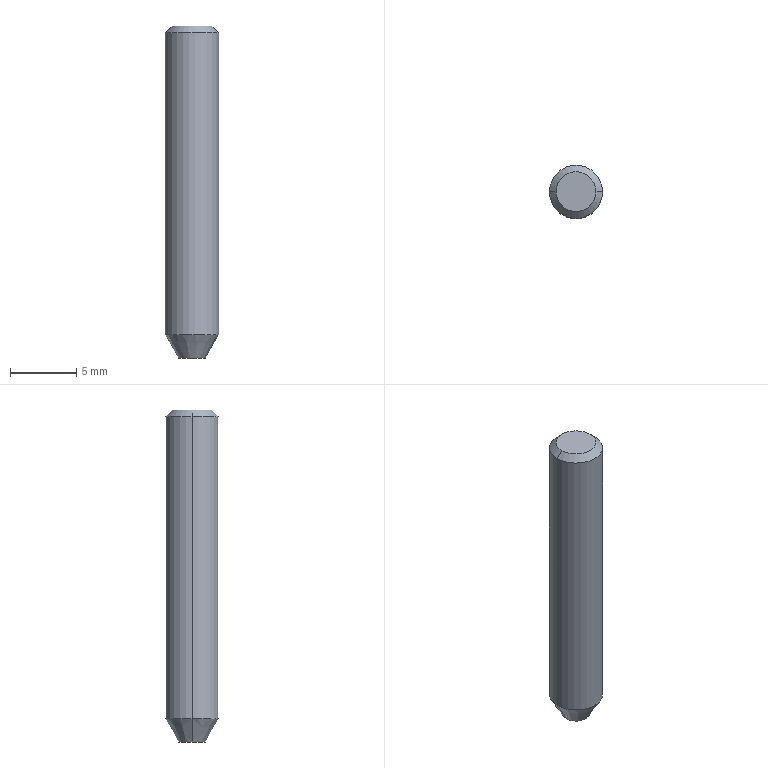Part | NX | features BREP 1 | 1 solid | 8 faces | box 4 x 4 x 25 mm | volume 303.65 mm3 | cone 4 | cylinder 2 | plane 2 | commonest cylinder face diameters 4 x2
STEP:
#1=CARTESIAN_POINT('',(1.5,0.,25.));
#2=VERTEX_POINT('',#1);
#3=CARTESIAN_POINT('',(-1.5,0.,25.));
#4=VERTEX_POINT('',#3);
#5=CARTESIAN_POINT('',(0.,0.,25.));
#6=DIRECTION('',(0.,0.,1.));
#7=DIRECTION('',(1.,0.,0.));
#8=AXIS2_PLACEMENT_3D('',#5,#6,#7);
#9=CIRCLE('',#8,1.5);
#10=EDGE_CURVE('',#2,#4,#9,.T.);
#11=ORIENTED_EDGE('',*,*,#10,.F.);
#12=CARTESIAN_POINT('',(2.,0.,24.5));
#13=VERTEX_POINT('',#12);
#14=CARTESIAN_POINT('',(1.5,0.,25.));
#15=DIRECTION('',(0.7071,0.,-0.7071));
#16=VECTOR('',#15,1000.);
#17=LINE('',#14,#16);
#18=EDGE_CURVE('',#2,#13,#17,.T.);
#19=ORIENTED_EDGE('',*,*,#18,.T.);
#20=CARTESIAN_POINT('',(-2.,0.,24.5));
#21=VERTEX_POINT('',#20);
#22=CARTESIAN_POINT('',(0.,0.,24.5));
#23=DIRECTION('',(0.,0.,-1.));
#24=DIRECTION('',(1.,0.,0.));
#25=AXIS2_PLACEMENT_3D('',#22,#23,#24);
#26=CIRCLE('',#25,2.);
#27=EDGE_CURVE('',#21,#13,#26,.T.);
#28=ORIENTED_EDGE('',*,*,#27,.F.);
#29=CARTESIAN_POINT('',(-1.5,0.,25.));
#30=DIRECTION('',(-0.7071,0.,-0.7071));
#31=VECTOR('',#30,1000.);
#32=LINE('',#29,#31);
#33=EDGE_CURVE('',#4,#21,#32,.T.);
#34=ORIENTED_EDGE('',*,*,#33,.F.);
#35=EDGE_LOOP('',(#11,#19,#28,#34));
#36=FACE_BOUND('',#35,.T.);
#37=CARTESIAN_POINT('',(0.,0.,25.));
#38=DIRECTION('',(0.,0.,-1.));
#39=DIRECTION('',(-1.,0.,0.));
#40=AXIS2_PLACEMENT_3D('',#37,#38,#39);
#41=CONICAL_SURFACE('',#40,1.5,0.7854);
#42=ADVANCED_FACE('',(#36),#41,.T.);
#43=CARTESIAN_POINT('',(-1.,0.,0.));
#44=VERTEX_POINT('',#43);
#45=CARTESIAN_POINT('',(1.,0.,0.));
#46=VERTEX_POINT('',#45);
#47=CARTESIAN_POINT('',(0.,0.,0.));
#48=DIRECTION('',(0.,0.,-1.));
#49=DIRECTION('',(1.,0.,0.));
#50=AXIS2_PLACEMENT_3D('',#47,#48,#49);
#51=CIRCLE('',#50,1.);
#52=EDGE_CURVE('',#44,#46,#51,.T.);
#53=ORIENTED_EDGE('',*,*,#52,.F.);
#54=CARTESIAN_POINT('',(-2.,0.,1.732));
#55=VERTEX_POINT('',#54);
#56=CARTESIAN_POINT('',(-2.,0.,1.732));
#57=DIRECTION('',(-0.5,0.,0.866));
#58=VECTOR('',#57,1000.);
#59=LINE('',#56,#58);
#60=EDGE_CURVE('',#55,#44,#59,.F.);
#61=ORIENTED_EDGE('',*,*,#60,.F.);
#62=CARTESIAN_POINT('',(2.,0.,1.732));
#63=VERTEX_POINT('',#62);
#64=CARTESIAN_POINT('',(0.,0.,1.732));
#65=DIRECTION('',(0.,0.,1.));
#66=DIRECTION('',(1.,0.,0.));
#67=AXIS2_PLACEMENT_3D('',#64,#65,#66);
#68=CIRCLE('',#67,2.);
#69=EDGE_CURVE('',#63,#55,#68,.T.);
#70=ORIENTED_EDGE('',*,*,#69,.F.);
#71=CARTESIAN_POINT('',(2.,0.,1.732));
#72=DIRECTION('',(0.5,0.,0.866));
#73=VECTOR('',#72,1000.);
#74=LINE('',#71,#73);
#75=EDGE_CURVE('',#63,#46,#74,.F.);
#76=ORIENTED_EDGE('',*,*,#75,.T.);
#77=EDGE_LOOP('',(#53,#61,#70,#76));
#78=FACE_BOUND('',#77,.T.);
#79=CARTESIAN_POINT('',(0.,0.,1.732));
#80=DIRECTION('',(0.,0.,1.));
#81=DIRECTION('',(1.,0.,0.));
#82=AXIS2_PLACEMENT_3D('',#79,#80,#81);
#83=CONICAL_SURFACE('',#82,2.,0.5236);
#84=ADVANCED_FACE('',(#78),#83,.T.);
#85=ORIENTED_EDGE('',*,*,#27,.T.);
#86=CARTESIAN_POINT('',(2.,0.,25.));
#87=DIRECTION('',(0.,0.,-1.));
#88=VECTOR('',#87,1000.);
#89=LINE('',#86,#88);
#90=EDGE_CURVE('',#13,#63,#89,.T.);
#91=ORIENTED_EDGE('',*,*,#90,.T.);
#92=ORIENTED_EDGE('',*,*,#69,.T.);
#93=CARTESIAN_POINT('',(-2.,0.,25.));
#94=DIRECTION('',(0.,0.,-1.));
#95=VECTOR('',#94,1000.);
#96=LINE('',#93,#95);
#97=EDGE_CURVE('',#21,#55,#96,.T.);
#98=ORIENTED_EDGE('',*,*,#97,.F.);
#99=EDGE_LOOP('',(#85,#91,#92,#98));
#100=FACE_BOUND('',#99,.T.);
#101=CARTESIAN_POINT('',(0.,0.,25.));
#102=DIRECTION('',(0.,0.,-1.));
#103=DIRECTION('',(-1.,0.,0.));
#104=AXIS2_PLACEMENT_3D('',#101,#102,#103);
#105=CYLINDRICAL_SURFACE('',#104,2.);
#106=ADVANCED_FACE('',(#100),#105,.T.);
#107=ORIENTED_EDGE('',*,*,#90,.F.);
#108=CARTESIAN_POINT('',(0.,0.,24.5));
#109=DIRECTION('',(0.,0.,-1.));
#110=DIRECTION('',(1.,0.,0.));
#111=AXIS2_PLACEMENT_3D('',#108,#109,#110);
#112=CIRCLE('',#111,2.);
#113=EDGE_CURVE('',#13,#21,#112,.T.);
#114=ORIENTED_EDGE('',*,*,#113,.T.);
#115=ORIENTED_EDGE('',*,*,#97,.T.);
#116=CARTESIAN_POINT('',(0.,0.,1.732));
#117=DIRECTION('',(0.,0.,1.));
#118=DIRECTION('',(1.,0.,0.));
#119=AXIS2_PLACEMENT_3D('',#116,#117,#118);
#120=CIRCLE('',#119,2.);
#121=EDGE_CURVE('',#55,#63,#120,.T.);
#122=ORIENTED_EDGE('',*,*,#121,.T.);
#123=EDGE_LOOP('',(#107,#114,#115,#122));
#124=FACE_BOUND('',#123,.T.);
#125=CARTESIAN_POINT('',(0.,0.,25.));
#126=DIRECTION('',(0.,0.,-1.));
#127=DIRECTION('',(-1.,0.,0.));
#128=AXIS2_PLACEMENT_3D('',#125,#126,#127);
#129=CYLINDRICAL_SURFACE('',#128,2.);
#130=ADVANCED_FACE('',(#124),#129,.T.);
#131=CARTESIAN_POINT('',(0.,0.,25.));
#132=DIRECTION('',(0.,0.,1.));
#133=DIRECTION('',(1.,0.,0.));
#134=AXIS2_PLACEMENT_3D('',#131,#132,#133);
#135=CIRCLE('',#134,1.5);
#136=EDGE_CURVE('',#4,#2,#135,.T.);
#137=ORIENTED_EDGE('',*,*,#136,.T.);
#138=ORIENTED_EDGE('',*,*,#10,.T.);
#139=EDGE_LOOP('',(#137,#138));
#140=FACE_BOUND('',#139,.T.);
#141=CARTESIAN_POINT('',(0.,0.,25.));
#142=DIRECTION('',(0.,0.,1.));
#143=DIRECTION('',(1.,0.,0.));
#144=AXIS2_PLACEMENT_3D('',#141,#142,#143);
#145=PLANE('',#144);
#146=ADVANCED_FACE('',(#140),#145,.T.);
#147=CARTESIAN_POINT('',(0.,0.,0.));
#148=DIRECTION('',(0.,0.,-1.));
#149=DIRECTION('',(1.,0.,0.));
#150=AXIS2_PLACEMENT_3D('',#147,#148,#149);
#151=CIRCLE('',#150,1.);
#152=EDGE_CURVE('',#46,#44,#151,.T.);
#153=ORIENTED_EDGE('',*,*,#152,.T.);
#154=ORIENTED_EDGE('',*,*,#52,.T.);
#155=EDGE_LOOP('',(#153,#154));
#156=FACE_BOUND('',#155,.T.);
#157=CARTESIAN_POINT('',(0.,0.,0.));
#158=DIRECTION('',(0.,0.,1.));
#159=DIRECTION('',(1.,0.,0.));
#160=AXIS2_PLACEMENT_3D('',#157,#158,#159);
#161=PLANE('',#160);
#162=ADVANCED_FACE('',(#156),#161,.F.);
#163=ORIENTED_EDGE('',*,*,#60,.T.);
#164=ORIENTED_EDGE('',*,*,#152,.F.);
#165=ORIENTED_EDGE('',*,*,#75,.F.);
#166=ORIENTED_EDGE('',*,*,#121,.F.);
#167=EDGE_LOOP('',(#163,#164,#165,#166));
#168=FACE_BOUND('',#167,.T.);
#169=CARTESIAN_POINT('',(0.,0.,1.732));
#170=DIRECTION('',(0.,0.,1.));
#171=DIRECTION('',(1.,0.,0.));
#172=AXIS2_PLACEMENT_3D('',#169,#170,#171);
#173=CONICAL_SURFACE('',#172,2.,0.5236);
#174=ADVANCED_FACE('',(#168),#173,.T.);
#175=ORIENTED_EDGE('',*,*,#18,.F.);
#176=ORIENTED_EDGE('',*,*,#136,.F.);
#177=ORIENTED_EDGE('',*,*,#33,.T.);
#178=ORIENTED_EDGE('',*,*,#113,.F.);
#179=EDGE_LOOP('',(#175,#176,#177,#178));
#180=FACE_BOUND('',#179,.T.);
#181=CARTESIAN_POINT('',(0.,0.,25.));
#182=DIRECTION('',(0.,0.,-1.));
#183=DIRECTION('',(-1.,0.,0.));
#184=AXIS2_PLACEMENT_3D('',#181,#182,#183);
#185=CONICAL_SURFACE('',#184,1.5,0.7854);
#186=ADVANCED_FACE('',(#180),#185,.T.);
#187=CLOSED_SHELL('',(#42,#84,#106,#130,#146,#162,#174,#186));
#188=MANIFOLD_SOLID_BREP('',#187);
#189=(LENGTH_UNIT()NAMED_UNIT(*)SI_UNIT(.MILLI.,.METRE.));
#190=UNCERTAINTY_MEASURE_WITH_UNIT(LENGTH_MEASURE(0.00001),#189,'','');
#191=(NAMED_UNIT(*)PLANE_ANGLE_UNIT()SI_UNIT($,.RADIAN.));
#192=(NAMED_UNIT(*)SI_UNIT($,.STERADIAN.)SOLID_ANGLE_UNIT());
#193=(GEOMETRIC_REPRESENTATION_CONTEXT(3)GLOBAL_UNCERTAINTY_ASSIGNED_CONTEXT((#190))GLOBAL_UNIT_ASSIGNED_CONTEXT((#189,#191,#192))REPRESENTATION_CONTEXT('',''));
#194=ADVANCED_BREP_SHAPE_REPRESENTATION('',(#188),#193);